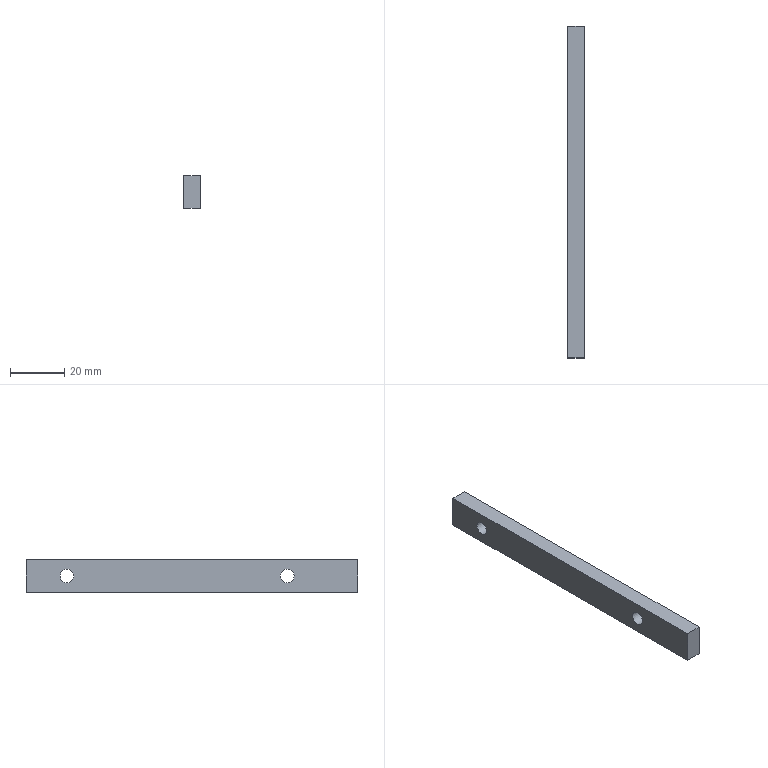Part | STEP file | 1-69.4 | 1 solid | 8 faces | box 6 x 122 x 12 mm | volume 8548 mm3 | plane 6 | cylinder 2 | commonest cylinder face diameters 5 x2
STEP:
#1=CARTESIAN_POINT('',(0.,0.,0.));
#2=DIRECTION('',(0.,0.,1.));
#3=DIRECTION('',(1.,0.,0.));
#4=AXIS2_PLACEMENT_3D('',#1,#2,#3);
#5=CARTESIAN_POINT('',(3.,-61.,-6.));
#6=VERTEX_POINT('',#5);
#7=CARTESIAN_POINT('',(3.,61.,-6.));
#8=VERTEX_POINT('',#7);
#9=CARTESIAN_POINT('',(3.,-61.,-6.));
#10=DIRECTION('',(0.,1.,0.));
#11=VECTOR('',#10,1.);
#12=LINE('',#9,#11);
#13=CARTESIAN_POINT('',(3.,0.,55.));
#14=DIRECTION('',(1.,0.,0.));
#15=DIRECTION('',(0.,1.,0.));
#16=AXIS2_PLACEMENT_3D('',#13,#14,#15);
#17=PLANE('',#16);
#18=CARTESIAN_POINT('',(-61.,-61.));
#19=DIRECTION('',(1.,0.));
#20=VECTOR('',#19,1.);
#21=LINE('',#18,#20);
#22=(GEOMETRIC_REPRESENTATION_CONTEXT(2)PARAMETRIC_REPRESENTATION_CONTEXT()REPRESENTATION_CONTEXT('',''));
#23=DEFINITIONAL_REPRESENTATION('',(#21),#22);
#24=PCURVE('',#17,#23);
#25=CARTESIAN_POINT('',(0.,0.,-6.));
#26=DIRECTION('',(0.,0.,1.));
#27=DIRECTION('',(0.,1.,0.));
#28=AXIS2_PLACEMENT_3D('',#25,#26,#27);
#29=PLANE('',#28);
#30=CARTESIAN_POINT('',(-61.,-3.));
#31=DIRECTION('',(1.,0.));
#32=VECTOR('',#31,1.);
#33=LINE('',#30,#32);
#34=(GEOMETRIC_REPRESENTATION_CONTEXT(2)PARAMETRIC_REPRESENTATION_CONTEXT()REPRESENTATION_CONTEXT('',''));
#35=DEFINITIONAL_REPRESENTATION('',(#33),#34);
#36=PCURVE('',#29,#35);
#37=SURFACE_CURVE('',#12,(#24,#36),.PCURVE_S1.);
#38=EDGE_CURVE('',#6,#8,#37,.T.);
#39=ORIENTED_EDGE('',*,*,#38,.T.);
#40=CARTESIAN_POINT('',(3.,61.,6.));
#41=VERTEX_POINT('',#40);
#42=CARTESIAN_POINT('',(3.,61.,-6.));
#43=DIRECTION('',(0.,0.,1.));
#44=VECTOR('',#43,1.);
#45=LINE('',#42,#44);
#46=CARTESIAN_POINT('',(61.,-61.));
#47=DIRECTION('',(0.,1.));
#48=VECTOR('',#47,1.);
#49=LINE('',#46,#48);
#50=(GEOMETRIC_REPRESENTATION_CONTEXT(2)PARAMETRIC_REPRESENTATION_CONTEXT()REPRESENTATION_CONTEXT('',''));
#51=DEFINITIONAL_REPRESENTATION('',(#49),#50);
#52=PCURVE('',#17,#51);
#53=CARTESIAN_POINT('',(0.,61.,0.));
#54=DIRECTION('',(0.,-1.,0.));
#55=DIRECTION('',(0.,0.,1.));
#56=AXIS2_PLACEMENT_3D('',#53,#54,#55);
#57=PLANE('',#56);
#58=CARTESIAN_POINT('',(-6.,-3.));
#59=DIRECTION('',(1.,0.));
#60=VECTOR('',#59,1.);
#61=LINE('',#58,#60);
#62=(GEOMETRIC_REPRESENTATION_CONTEXT(2)PARAMETRIC_REPRESENTATION_CONTEXT()REPRESENTATION_CONTEXT('',''));
#63=DEFINITIONAL_REPRESENTATION('',(#61),#62);
#64=PCURVE('',#57,#63);
#65=SURFACE_CURVE('',#45,(#52,#64),.PCURVE_S1.);
#66=EDGE_CURVE('',#8,#41,#65,.T.);
#67=ORIENTED_EDGE('',*,*,#66,.T.);
#68=CARTESIAN_POINT('',(3.,-61.,6.));
#69=VERTEX_POINT('',#68);
#70=CARTESIAN_POINT('',(3.,61.,6.));
#71=DIRECTION('',(0.,-1.,0.));
#72=VECTOR('',#71,1.);
#73=LINE('',#70,#72);
#74=CARTESIAN_POINT('',(61.,-49.));
#75=DIRECTION('',(-1.,0.));
#76=VECTOR('',#75,1.);
#77=LINE('',#74,#76);
#78=(GEOMETRIC_REPRESENTATION_CONTEXT(2)PARAMETRIC_REPRESENTATION_CONTEXT()REPRESENTATION_CONTEXT('',''));
#79=DEFINITIONAL_REPRESENTATION('',(#77),#78);
#80=PCURVE('',#17,#79);
#81=CARTESIAN_POINT('',(0.,0.,6.));
#82=DIRECTION('',(0.,0.,-1.));
#83=DIRECTION('',(0.,-1.,0.));
#84=AXIS2_PLACEMENT_3D('',#81,#82,#83);
#85=PLANE('',#84);
#86=CARTESIAN_POINT('',(-61.,-3.));
#87=DIRECTION('',(1.,0.));
#88=VECTOR('',#87,1.);
#89=LINE('',#86,#88);
#90=(GEOMETRIC_REPRESENTATION_CONTEXT(2)PARAMETRIC_REPRESENTATION_CONTEXT()REPRESENTATION_CONTEXT('',''));
#91=DEFINITIONAL_REPRESENTATION('',(#89),#90);
#92=PCURVE('',#85,#91);
#93=SURFACE_CURVE('',#73,(#80,#92),.PCURVE_S1.);
#94=EDGE_CURVE('',#41,#69,#93,.T.);
#95=ORIENTED_EDGE('',*,*,#94,.T.);
#96=CARTESIAN_POINT('',(3.,-61.,6.));
#97=DIRECTION('',(0.,0.,-1.));
#98=VECTOR('',#97,1.);
#99=LINE('',#96,#98);
#100=CARTESIAN_POINT('',(-61.,-49.));
#101=DIRECTION('',(0.,-1.));
#102=VECTOR('',#101,1.);
#103=LINE('',#100,#102);
#104=(GEOMETRIC_REPRESENTATION_CONTEXT(2)PARAMETRIC_REPRESENTATION_CONTEXT()REPRESENTATION_CONTEXT('',''));
#105=DEFINITIONAL_REPRESENTATION('',(#103),#104);
#106=PCURVE('',#17,#105);
#107=CARTESIAN_POINT('',(0.,-61.,0.));
#108=DIRECTION('',(0.,1.,0.));
#109=DIRECTION('',(0.,0.,-1.));
#110=AXIS2_PLACEMENT_3D('',#107,#108,#109);
#111=PLANE('',#110);
#112=CARTESIAN_POINT('',(-6.,-3.));
#113=DIRECTION('',(1.,0.));
#114=VECTOR('',#113,1.);
#115=LINE('',#112,#114);
#116=(GEOMETRIC_REPRESENTATION_CONTEXT(2)PARAMETRIC_REPRESENTATION_CONTEXT()REPRESENTATION_CONTEXT('',''));
#117=DEFINITIONAL_REPRESENTATION('',(#115),#116);
#118=PCURVE('',#111,#117);
#119=SURFACE_CURVE('',#99,(#106,#118),.PCURVE_S1.);
#120=EDGE_CURVE('',#69,#6,#119,.T.);
#121=ORIENTED_EDGE('',*,*,#120,.T.);
#122=EDGE_LOOP('',(#39,#67,#95,#121));
#123=FACE_BOUND('',#122,.T.);
#124=CARTESIAN_POINT('',(3.,-32.5,0.));
#125=VERTEX_POINT('',#124);
#126=CARTESIAN_POINT('',(3.,-35.,0.));
#127=DIRECTION('',(-1.,0.,0.));
#128=DIRECTION('',(0.,1.,0.));
#129=AXIS2_PLACEMENT_3D('',#126,#127,#128);
#130=CIRCLE('',#129,2.5);
#131=CARTESIAN_POINT('',(-32.5,-55.));
#132=CARTESIAN_POINT('',(-32.5,-59.33));
#133=CARTESIAN_POINT('',(-36.25,-57.165));
#134=CARTESIAN_POINT('',(-40.,-55.));
#135=CARTESIAN_POINT('',(-36.25,-52.835));
#136=CARTESIAN_POINT('',(-32.5,-50.67));
#137=CARTESIAN_POINT('',(-32.5,-55.));
#138=(BOUNDED_CURVE()B_SPLINE_CURVE(2,(#131,#132,#133,#134,#135,#136,#137),.UNSPECIFIED.,.T.,.F.)B_SPLINE_CURVE_WITH_KNOTS((1,2,2,2,2,1),(-2.094,0.,2.094,4.189,6.283,8.378),.UNSPECIFIED.)CURVE()GEOMETRIC_REPRESENTATION_ITEM()RATIONAL_B_SPLINE_CURVE((1.,0.5,1.,0.5,1.,0.5,1.))REPRESENTATION_ITEM(''));
#139=(GEOMETRIC_REPRESENTATION_CONTEXT(2)PARAMETRIC_REPRESENTATION_CONTEXT()REPRESENTATION_CONTEXT('',''));
#140=DEFINITIONAL_REPRESENTATION('',(#138),#139);
#141=PCURVE('',#17,#140);
#142=CARTESIAN_POINT('',(3.,-35.,0.));
#143=DIRECTION('',(-1.,0.,0.));
#144=DIRECTION('',(0.,1.,0.));
#145=AXIS2_PLACEMENT_3D('',#142,#143,#144);
#146=CYLINDRICAL_SURFACE('',#145,2.5);
#147=CARTESIAN_POINT('',(0.,0.));
#148=DIRECTION('',(1.,0.));
#149=VECTOR('',#148,1.);
#150=LINE('',#147,#149);
#151=(GEOMETRIC_REPRESENTATION_CONTEXT(2)PARAMETRIC_REPRESENTATION_CONTEXT()REPRESENTATION_CONTEXT('',''));
#152=DEFINITIONAL_REPRESENTATION('',(#150),#151);
#153=PCURVE('',#146,#152);
#154=SURFACE_CURVE('',#130,(#141,#153),.PCURVE_S1.);
#155=EDGE_CURVE('',#125,#125,#154,.T.);
#156=ORIENTED_EDGE('',*,*,#155,.T.);
#157=EDGE_LOOP('',(#156));
#158=FACE_BOUND('',#157,.T.);
#159=CARTESIAN_POINT('',(3.,48.5,0.));
#160=VERTEX_POINT('',#159);
#161=CARTESIAN_POINT('',(3.,46.,0.));
#162=DIRECTION('',(-1.,0.,0.));
#163=DIRECTION('',(0.,1.,0.));
#164=AXIS2_PLACEMENT_3D('',#161,#162,#163);
#165=CIRCLE('',#164,2.5);
#166=CARTESIAN_POINT('',(48.5,-55.));
#167=CARTESIAN_POINT('',(48.5,-59.33));
#168=CARTESIAN_POINT('',(44.75,-57.165));
#169=CARTESIAN_POINT('',(41.,-55.));
#170=CARTESIAN_POINT('',(44.75,-52.835));
#171=CARTESIAN_POINT('',(48.5,-50.67));
#172=CARTESIAN_POINT('',(48.5,-55.));
#173=(BOUNDED_CURVE()B_SPLINE_CURVE(2,(#166,#167,#168,#169,#170,#171,#172),.UNSPECIFIED.,.T.,.F.)B_SPLINE_CURVE_WITH_KNOTS((1,2,2,2,2,1),(-2.094,0.,2.094,4.189,6.283,8.378),.UNSPECIFIED.)CURVE()GEOMETRIC_REPRESENTATION_ITEM()RATIONAL_B_SPLINE_CURVE((1.,0.5,1.,0.5,1.,0.5,1.))REPRESENTATION_ITEM(''));
#174=(GEOMETRIC_REPRESENTATION_CONTEXT(2)PARAMETRIC_REPRESENTATION_CONTEXT()REPRESENTATION_CONTEXT('',''));
#175=DEFINITIONAL_REPRESENTATION('',(#173),#174);
#176=PCURVE('',#17,#175);
#177=CARTESIAN_POINT('',(3.,46.,0.));
#178=DIRECTION('',(-1.,0.,0.));
#179=DIRECTION('',(0.,1.,0.));
#180=AXIS2_PLACEMENT_3D('',#177,#178,#179);
#181=CYLINDRICAL_SURFACE('',#180,2.5);
#182=CARTESIAN_POINT('',(0.,0.));
#183=DIRECTION('',(1.,0.));
#184=VECTOR('',#183,1.);
#185=LINE('',#182,#184);
#186=(GEOMETRIC_REPRESENTATION_CONTEXT(2)PARAMETRIC_REPRESENTATION_CONTEXT()REPRESENTATION_CONTEXT('',''));
#187=DEFINITIONAL_REPRESENTATION('',(#185),#186);
#188=PCURVE('',#181,#187);
#189=SURFACE_CURVE('',#165,(#176,#188),.PCURVE_S1.);
#190=EDGE_CURVE('',#160,#160,#189,.T.);
#191=ORIENTED_EDGE('',*,*,#190,.T.);
#192=EDGE_LOOP('',(#191));
#193=FACE_BOUND('',#192,.T.);
#194=ADVANCED_FACE('',(#123,#158,#193),#17,.T.);
#195=CARTESIAN_POINT('',(-3.,-61.,-6.));
#196=VERTEX_POINT('',#195);
#197=CARTESIAN_POINT('',(-3.,61.,-6.));
#198=VERTEX_POINT('',#197);
#199=CARTESIAN_POINT('',(-3.,-61.,-6.));
#200=DIRECTION('',(0.,1.,0.));
#201=VECTOR('',#200,1.);
#202=LINE('',#199,#201);
#203=CARTESIAN_POINT('',(-3.,0.,55.));
#204=DIRECTION('',(1.,0.,0.));
#205=DIRECTION('',(0.,1.,0.));
#206=AXIS2_PLACEMENT_3D('',#203,#204,#205);
#207=PLANE('',#206);
#208=CARTESIAN_POINT('',(-61.,-61.));
#209=DIRECTION('',(1.,0.));
#210=VECTOR('',#209,1.);
#211=LINE('',#208,#210);
#212=(GEOMETRIC_REPRESENTATION_CONTEXT(2)PARAMETRIC_REPRESENTATION_CONTEXT()REPRESENTATION_CONTEXT('',''));
#213=DEFINITIONAL_REPRESENTATION('',(#211),#212);
#214=PCURVE('',#207,#213);
#215=CARTESIAN_POINT('',(-61.,3.));
#216=DIRECTION('',(1.,0.));
#217=VECTOR('',#216,1.);
#218=LINE('',#215,#217);
#219=(GEOMETRIC_REPRESENTATION_CONTEXT(2)PARAMETRIC_REPRESENTATION_CONTEXT()REPRESENTATION_CONTEXT('',''));
#220=DEFINITIONAL_REPRESENTATION('',(#218),#219);
#221=PCURVE('',#29,#220);
#222=SURFACE_CURVE('',#202,(#214,#221),.PCURVE_S1.);
#223=EDGE_CURVE('',#196,#198,#222,.T.);
#224=ORIENTED_EDGE('',*,*,#223,.T.);
#225=CARTESIAN_POINT('',(-3.,61.,6.));
#226=VERTEX_POINT('',#225);
#227=CARTESIAN_POINT('',(-3.,61.,-6.));
#228=DIRECTION('',(0.,0.,1.));
#229=VECTOR('',#228,1.);
#230=LINE('',#227,#229);
#231=CARTESIAN_POINT('',(61.,-61.));
#232=DIRECTION('',(0.,1.));
#233=VECTOR('',#232,1.);
#234=LINE('',#231,#233);
#235=(GEOMETRIC_REPRESENTATION_CONTEXT(2)PARAMETRIC_REPRESENTATION_CONTEXT()REPRESENTATION_CONTEXT('',''));
#236=DEFINITIONAL_REPRESENTATION('',(#234),#235);
#237=PCURVE('',#207,#236);
#238=CARTESIAN_POINT('',(-6.,3.));
#239=DIRECTION('',(1.,0.));
#240=VECTOR('',#239,1.);
#241=LINE('',#238,#240);
#242=(GEOMETRIC_REPRESENTATION_CONTEXT(2)PARAMETRIC_REPRESENTATION_CONTEXT()REPRESENTATION_CONTEXT('',''));
#243=DEFINITIONAL_REPRESENTATION('',(#241),#242);
#244=PCURVE('',#57,#243);
#245=SURFACE_CURVE('',#230,(#237,#244),.PCURVE_S1.);
#246=EDGE_CURVE('',#198,#226,#245,.T.);
#247=ORIENTED_EDGE('',*,*,#246,.T.);
#248=CARTESIAN_POINT('',(-3.,-61.,6.));
#249=VERTEX_POINT('',#248);
#250=CARTESIAN_POINT('',(-3.,61.,6.));
#251=DIRECTION('',(0.,-1.,0.));
#252=VECTOR('',#251,1.);
#253=LINE('',#250,#252);
#254=CARTESIAN_POINT('',(61.,-49.));
#255=DIRECTION('',(-1.,0.));
#256=VECTOR('',#255,1.);
#257=LINE('',#254,#256);
#258=(GEOMETRIC_REPRESENTATION_CONTEXT(2)PARAMETRIC_REPRESENTATION_CONTEXT()REPRESENTATION_CONTEXT('',''));
#259=DEFINITIONAL_REPRESENTATION('',(#257),#258);
#260=PCURVE('',#207,#259);
#261=CARTESIAN_POINT('',(-61.,3.));
#262=DIRECTION('',(1.,0.));
#263=VECTOR('',#262,1.);
#264=LINE('',#261,#263);
#265=(GEOMETRIC_REPRESENTATION_CONTEXT(2)PARAMETRIC_REPRESENTATION_CONTEXT()REPRESENTATION_CONTEXT('',''));
#266=DEFINITIONAL_REPRESENTATION('',(#264),#265);
#267=PCURVE('',#85,#266);
#268=SURFACE_CURVE('',#253,(#260,#267),.PCURVE_S1.);
#269=EDGE_CURVE('',#226,#249,#268,.T.);
#270=ORIENTED_EDGE('',*,*,#269,.T.);
#271=CARTESIAN_POINT('',(-3.,-61.,6.));
#272=DIRECTION('',(0.,0.,-1.));
#273=VECTOR('',#272,1.);
#274=LINE('',#271,#273);
#275=CARTESIAN_POINT('',(-61.,-49.));
#276=DIRECTION('',(0.,-1.));
#277=VECTOR('',#276,1.);
#278=LINE('',#275,#277);
#279=(GEOMETRIC_REPRESENTATION_CONTEXT(2)PARAMETRIC_REPRESENTATION_CONTEXT()REPRESENTATION_CONTEXT('',''));
#280=DEFINITIONAL_REPRESENTATION('',(#278),#279);
#281=PCURVE('',#207,#280);
#282=CARTESIAN_POINT('',(-6.,3.));
#283=DIRECTION('',(1.,0.));
#284=VECTOR('',#283,1.);
#285=LINE('',#282,#284);
#286=(GEOMETRIC_REPRESENTATION_CONTEXT(2)PARAMETRIC_REPRESENTATION_CONTEXT()REPRESENTATION_CONTEXT('',''));
#287=DEFINITIONAL_REPRESENTATION('',(#285),#286);
#288=PCURVE('',#111,#287);
#289=SURFACE_CURVE('',#274,(#281,#288),.PCURVE_S1.);
#290=EDGE_CURVE('',#249,#196,#289,.T.);
#291=ORIENTED_EDGE('',*,*,#290,.T.);
#292=EDGE_LOOP('',(#224,#247,#270,#291));
#293=FACE_BOUND('',#292,.F.);
#294=CARTESIAN_POINT('',(-3.,-32.5,0.));
#295=VERTEX_POINT('',#294);
#296=CARTESIAN_POINT('',(-3.,-35.,0.));
#297=DIRECTION('',(-1.,0.,0.));
#298=DIRECTION('',(0.,1.,0.));
#299=AXIS2_PLACEMENT_3D('',#296,#297,#298);
#300=CIRCLE('',#299,2.5);
#301=CARTESIAN_POINT('',(-32.5,-55.));
#302=CARTESIAN_POINT('',(-32.5,-59.33));
#303=CARTESIAN_POINT('',(-36.25,-57.165));
#304=CARTESIAN_POINT('',(-40.,-55.));
#305=CARTESIAN_POINT('',(-36.25,-52.835));
#306=CARTESIAN_POINT('',(-32.5,-50.67));
#307=CARTESIAN_POINT('',(-32.5,-55.));
#308=(BOUNDED_CURVE()B_SPLINE_CURVE(2,(#301,#302,#303,#304,#305,#306,#307),.UNSPECIFIED.,.T.,.F.)B_SPLINE_CURVE_WITH_KNOTS((1,2,2,2,2,1),(-2.094,0.,2.094,4.189,6.283,8.378),.UNSPECIFIED.)CURVE()GEOMETRIC_REPRESENTATION_ITEM()RATIONAL_B_SPLINE_CURVE((1.,0.5,1.,0.5,1.,0.5,1.))REPRESENTATION_ITEM(''));
#309=(GEOMETRIC_REPRESENTATION_CONTEXT(2)PARAMETRIC_REPRESENTATION_CONTEXT()REPRESENTATION_CONTEXT('',''));
#310=DEFINITIONAL_REPRESENTATION('',(#308),#309);
#311=PCURVE('',#207,#310);
#312=CARTESIAN_POINT('',(0.,6.));
#313=DIRECTION('',(1.,0.));
#314=VECTOR('',#313,1.);
#315=LINE('',#312,#314);
#316=(GEOMETRIC_REPRESENTATION_CONTEXT(2)PARAMETRIC_REPRESENTATION_CONTEXT()REPRESENTATION_CONTEXT('',''));
#317=DEFINITIONAL_REPRESENTATION('',(#315),#316);
#318=PCURVE('',#146,#317);
#319=SURFACE_CURVE('',#300,(#311,#318),.PCURVE_S1.);
#320=EDGE_CURVE('',#295,#295,#319,.T.);
#321=ORIENTED_EDGE('',*,*,#320,.T.);
#322=EDGE_LOOP('',(#321));
#323=FACE_BOUND('',#322,.F.);
#324=CARTESIAN_POINT('',(-3.,48.5,0.));
#325=VERTEX_POINT('',#324);
#326=CARTESIAN_POINT('',(-3.,46.,0.));
#327=DIRECTION('',(-1.,0.,0.));
#328=DIRECTION('',(0.,1.,0.));
#329=AXIS2_PLACEMENT_3D('',#326,#327,#328);
#330=CIRCLE('',#329,2.5);
#331=CARTESIAN_POINT('',(48.5,-55.));
#332=CARTESIAN_POINT('',(48.5,-59.33));
#333=CARTESIAN_POINT('',(44.75,-57.165));
#334=CARTESIAN_POINT('',(41.,-55.));
#335=CARTESIAN_POINT('',(44.75,-52.835));
#336=CARTESIAN_POINT('',(48.5,-50.67));
#337=CARTESIAN_POINT('',(48.5,-55.));
#338=(BOUNDED_CURVE()B_SPLINE_CURVE(2,(#331,#332,#333,#334,#335,#336,#337),.UNSPECIFIED.,.T.,.F.)B_SPLINE_CURVE_WITH_KNOTS((1,2,2,2,2,1),(-2.094,0.,2.094,4.189,6.283,8.378),.UNSPECIFIED.)CURVE()GEOMETRIC_REPRESENTATION_ITEM()RATIONAL_B_SPLINE_CURVE((1.,0.5,1.,0.5,1.,0.5,1.))REPRESENTATION_ITEM(''));
#339=(GEOMETRIC_REPRESENTATION_CONTEXT(2)PARAMETRIC_REPRESENTATION_CONTEXT()REPRESENTATION_CONTEXT('',''));
#340=DEFINITIONAL_REPRESENTATION('',(#338),#339);
#341=PCURVE('',#207,#340);
#342=CARTESIAN_POINT('',(0.,6.));
#343=DIRECTION('',(1.,0.));
#344=VECTOR('',#343,1.);
#345=LINE('',#342,#344);
#346=(GEOMETRIC_REPRESENTATION_CONTEXT(2)PARAMETRIC_REPRESENTATION_CONTEXT()REPRESENTATION_CONTEXT('',''));
#347=DEFINITIONAL_REPRESENTATION('',(#345),#346);
#348=PCURVE('',#181,#347);
#349=SURFACE_CURVE('',#330,(#341,#348),.PCURVE_S1.);
#350=EDGE_CURVE('',#325,#325,#349,.T.);
#351=ORIENTED_EDGE('',*,*,#350,.T.);
#352=EDGE_LOOP('',(#351));
#353=FACE_BOUND('',#352,.F.);
#354=ADVANCED_FACE('',(#293,#323,#353),#207,.F.);
#355=ORIENTED_EDGE('',*,*,#38,.T.);
#356=CARTESIAN_POINT('',(3.,61.,-6.));
#357=DIRECTION('',(-1.,0.,0.));
#358=VECTOR('',#357,1.);
#359=LINE('',#356,#358);
#360=CARTESIAN_POINT('',(61.,-3.));
#361=DIRECTION('',(0.,1.));
#362=VECTOR('',#361,1.);
#363=LINE('',#360,#362);
#364=(GEOMETRIC_REPRESENTATION_CONTEXT(2)PARAMETRIC_REPRESENTATION_CONTEXT()REPRESENTATION_CONTEXT('',''));
#365=DEFINITIONAL_REPRESENTATION('',(#363),#364);
#366=PCURVE('',#29,#365);
#367=CARTESIAN_POINT('',(-6.,-3.));
#368=DIRECTION('',(0.,1.));
#369=VECTOR('',#368,1.);
#370=LINE('',#367,#369);
#371=(GEOMETRIC_REPRESENTATION_CONTEXT(2)PARAMETRIC_REPRESENTATION_CONTEXT()REPRESENTATION_CONTEXT('',''));
#372=DEFINITIONAL_REPRESENTATION('',(#370),#371);
#373=PCURVE('',#57,#372);
#374=SURFACE_CURVE('',#359,(#366,#373),.PCURVE_S1.);
#375=EDGE_CURVE('',#8,#198,#374,.T.);
#376=ORIENTED_EDGE('',*,*,#375,.T.);
#377=ORIENTED_EDGE('',*,*,#223,.F.);
#378=CARTESIAN_POINT('',(3.,-61.,-6.));
#379=DIRECTION('',(-1.,0.,0.));
#380=VECTOR('',#379,1.);
#381=LINE('',#378,#380);
#382=CARTESIAN_POINT('',(-61.,-3.));
#383=DIRECTION('',(0.,1.));
#384=VECTOR('',#383,1.);
#385=LINE('',#382,#384);
#386=(GEOMETRIC_REPRESENTATION_CONTEXT(2)PARAMETRIC_REPRESENTATION_CONTEXT()REPRESENTATION_CONTEXT('',''));
#387=DEFINITIONAL_REPRESENTATION('',(#385),#386);
#388=PCURVE('',#29,#387);
#389=CARTESIAN_POINT('',(6.,-3.));
#390=DIRECTION('',(0.,1.));
#391=VECTOR('',#390,1.);
#392=LINE('',#389,#391);
#393=(GEOMETRIC_REPRESENTATION_CONTEXT(2)PARAMETRIC_REPRESENTATION_CONTEXT()REPRESENTATION_CONTEXT('',''));
#394=DEFINITIONAL_REPRESENTATION('',(#392),#393);
#395=PCURVE('',#111,#394);
#396=SURFACE_CURVE('',#381,(#388,#395),.PCURVE_S1.);
#397=EDGE_CURVE('',#6,#196,#396,.T.);
#398=ORIENTED_EDGE('',*,*,#397,.F.);
#399=EDGE_LOOP('',(#355,#376,#377,#398));
#400=FACE_BOUND('',#399,.F.);
#401=ADVANCED_FACE('',(#400),#29,.F.);
#402=ORIENTED_EDGE('',*,*,#66,.T.);
#403=CARTESIAN_POINT('',(3.,61.,6.));
#404=DIRECTION('',(-1.,0.,0.));
#405=VECTOR('',#404,1.);
#406=LINE('',#403,#405);
#407=CARTESIAN_POINT('',(6.,-3.));
#408=DIRECTION('',(0.,1.));
#409=VECTOR('',#408,1.);
#410=LINE('',#407,#409);
#411=(GEOMETRIC_REPRESENTATION_CONTEXT(2)PARAMETRIC_REPRESENTATION_CONTEXT()REPRESENTATION_CONTEXT('',''));
#412=DEFINITIONAL_REPRESENTATION('',(#410),#411);
#413=PCURVE('',#57,#412);
#414=CARTESIAN_POINT('',(-61.,-3.));
#415=DIRECTION('',(0.,1.));
#416=VECTOR('',#415,1.);
#417=LINE('',#414,#416);
#418=(GEOMETRIC_REPRESENTATION_CONTEXT(2)PARAMETRIC_REPRESENTATION_CONTEXT()REPRESENTATION_CONTEXT('',''));
#419=DEFINITIONAL_REPRESENTATION('',(#417),#418);
#420=PCURVE('',#85,#419);
#421=SURFACE_CURVE('',#406,(#413,#420),.PCURVE_S1.);
#422=EDGE_CURVE('',#41,#226,#421,.T.);
#423=ORIENTED_EDGE('',*,*,#422,.T.);
#424=ORIENTED_EDGE('',*,*,#246,.F.);
#425=ORIENTED_EDGE('',*,*,#375,.F.);
#426=EDGE_LOOP('',(#402,#423,#424,#425));
#427=FACE_BOUND('',#426,.F.);
#428=ADVANCED_FACE('',(#427),#57,.F.);
#429=ORIENTED_EDGE('',*,*,#94,.T.);
#430=CARTESIAN_POINT('',(3.,-61.,6.));
#431=DIRECTION('',(-1.,0.,0.));
#432=VECTOR('',#431,1.);
#433=LINE('',#430,#432);
#434=CARTESIAN_POINT('',(61.,-3.));
#435=DIRECTION('',(0.,1.));
#436=VECTOR('',#435,1.);
#437=LINE('',#434,#436);
#438=(GEOMETRIC_REPRESENTATION_CONTEXT(2)PARAMETRIC_REPRESENTATION_CONTEXT()REPRESENTATION_CONTEXT('',''));
#439=DEFINITIONAL_REPRESENTATION('',(#437),#438);
#440=PCURVE('',#85,#439);
#441=CARTESIAN_POINT('',(-6.,-3.));
#442=DIRECTION('',(0.,1.));
#443=VECTOR('',#442,1.);
#444=LINE('',#441,#443);
#445=(GEOMETRIC_REPRESENTATION_CONTEXT(2)PARAMETRIC_REPRESENTATION_CONTEXT()REPRESENTATION_CONTEXT('',''));
#446=DEFINITIONAL_REPRESENTATION('',(#444),#445);
#447=PCURVE('',#111,#446);
#448=SURFACE_CURVE('',#433,(#440,#447),.PCURVE_S1.);
#449=EDGE_CURVE('',#69,#249,#448,.T.);
#450=ORIENTED_EDGE('',*,*,#449,.T.);
#451=ORIENTED_EDGE('',*,*,#269,.F.);
#452=ORIENTED_EDGE('',*,*,#422,.F.);
#453=EDGE_LOOP('',(#429,#450,#451,#452));
#454=FACE_BOUND('',#453,.F.);
#455=ADVANCED_FACE('',(#454),#85,.F.);
#456=ORIENTED_EDGE('',*,*,#120,.T.);
#457=ORIENTED_EDGE('',*,*,#397,.T.);
#458=ORIENTED_EDGE('',*,*,#290,.F.);
#459=ORIENTED_EDGE('',*,*,#449,.F.);
#460=EDGE_LOOP('',(#456,#457,#458,#459));
#461=FACE_BOUND('',#460,.F.);
#462=ADVANCED_FACE('',(#461),#111,.F.);
#463=ORIENTED_EDGE('',*,*,#155,.T.);
#464=CARTESIAN_POINT('',(3.,-32.5,0.));
#465=DIRECTION('',(-1.,0.,0.));
#466=VECTOR('',#465,1.);
#467=LINE('',#464,#466);
#468=CARTESIAN_POINT('',(6.283,0.));
#469=DIRECTION('',(0.,1.));
#470=VECTOR('',#469,1.);
#471=LINE('',#468,#470);
#472=(GEOMETRIC_REPRESENTATION_CONTEXT(2)PARAMETRIC_REPRESENTATION_CONTEXT()REPRESENTATION_CONTEXT('',''));
#473=DEFINITIONAL_REPRESENTATION('',(#471),#472);
#474=PCURVE('',#146,#473);
#475=CARTESIAN_POINT('',(0.,0.));
#476=DIRECTION('',(0.,1.));
#477=VECTOR('',#476,1.);
#478=LINE('',#475,#477);
#479=(GEOMETRIC_REPRESENTATION_CONTEXT(2)PARAMETRIC_REPRESENTATION_CONTEXT()REPRESENTATION_CONTEXT('',''));
#480=DEFINITIONAL_REPRESENTATION('',(#478),#479);
#481=PCURVE('',#146,#480);
#482=SEAM_CURVE('',#467,(#474,#481),.PCURVE_S1.);
#483=EDGE_CURVE('',#125,#295,#482,.T.);
#484=ORIENTED_EDGE('',*,*,#483,.T.);
#485=ORIENTED_EDGE('',*,*,#320,.F.);
#486=ORIENTED_EDGE('',*,*,#483,.F.);
#487=EDGE_LOOP('',(#463,#484,#485,#486));
#488=FACE_BOUND('',#487,.F.);
#489=ADVANCED_FACE('',(#488),#146,.F.);
#490=ORIENTED_EDGE('',*,*,#190,.T.);
#491=CARTESIAN_POINT('',(3.,48.5,0.));
#492=DIRECTION('',(-1.,0.,0.));
#493=VECTOR('',#492,1.);
#494=LINE('',#491,#493);
#495=CARTESIAN_POINT('',(6.283,0.));
#496=DIRECTION('',(0.,1.));
#497=VECTOR('',#496,1.);
#498=LINE('',#495,#497);
#499=(GEOMETRIC_REPRESENTATION_CONTEXT(2)PARAMETRIC_REPRESENTATION_CONTEXT()REPRESENTATION_CONTEXT('',''));
#500=DEFINITIONAL_REPRESENTATION('',(#498),#499);
#501=PCURVE('',#181,#500);
#502=CARTESIAN_POINT('',(0.,0.));
#503=DIRECTION('',(0.,1.));
#504=VECTOR('',#503,1.);
#505=LINE('',#502,#504);
#506=(GEOMETRIC_REPRESENTATION_CONTEXT(2)PARAMETRIC_REPRESENTATION_CONTEXT()REPRESENTATION_CONTEXT('',''));
#507=DEFINITIONAL_REPRESENTATION('',(#505),#506);
#508=PCURVE('',#181,#507);
#509=SEAM_CURVE('',#494,(#501,#508),.PCURVE_S1.);
#510=EDGE_CURVE('',#160,#325,#509,.T.);
#511=ORIENTED_EDGE('',*,*,#510,.T.);
#512=ORIENTED_EDGE('',*,*,#350,.F.);
#513=ORIENTED_EDGE('',*,*,#510,.F.);
#514=EDGE_LOOP('',(#490,#511,#512,#513));
#515=FACE_BOUND('',#514,.F.);
#516=ADVANCED_FACE('',(#515),#181,.F.);
#517=CLOSED_SHELL('',(#194,#354,#401,#428,#455,#462,#489,#516));
#518=MANIFOLD_SOLID_BREP('',#517);
#519=(LENGTH_UNIT()NAMED_UNIT(*)SI_UNIT(.MILLI.,.METRE.));
#520=UNCERTAINTY_MEASURE_WITH_UNIT(LENGTH_MEASURE(0.0000001),#519,'','');
#521=(NAMED_UNIT(*)PLANE_ANGLE_UNIT()SI_UNIT($,.RADIAN.));
#522=(NAMED_UNIT(*)SI_UNIT($,.STERADIAN.)SOLID_ANGLE_UNIT());
#523=(GEOMETRIC_REPRESENTATION_CONTEXT(3)GLOBAL_UNCERTAINTY_ASSIGNED_CONTEXT((#520))GLOBAL_UNIT_ASSIGNED_CONTEXT((#519,#521,#522))REPRESENTATION_CONTEXT('',''));
#524=ADVANCED_BREP_SHAPE_REPRESENTATION('',(#4,#518),#523);